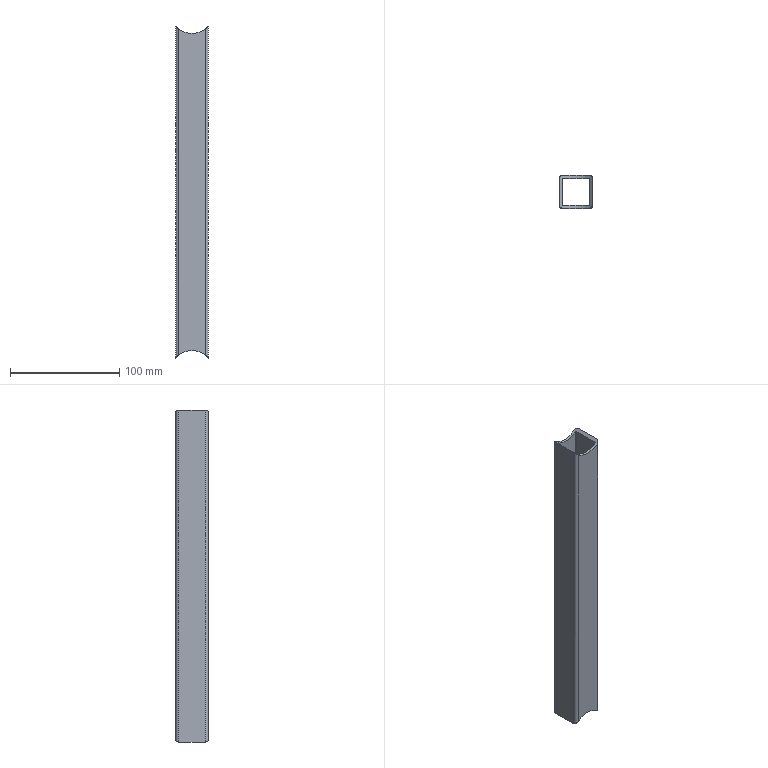Part | SolidWorks | features ExtruThin 1, ICE 1 | 1 solid | 19 faces | box 30 x 30 x 303.542 mm | volume 79870 mm3 | cylinder 11 | plane 8 | commonest cylinder face diameters 0.4 x4 5.4 x4 40 x3
STEP:
#1=CARTESIAN_POINT('',(0.,-15.,-145.));
#2=VERTEX_POINT('',#1);
#3=CARTESIAN_POINT('',(12.3,-15.,-149.229));
#4=VERTEX_POINT('',#3);
#5=CARTESIAN_POINT('',(0.,-15.,-165.));
#6=DIRECTION('',(0.,1.,0.));
#7=DIRECTION('',(0.,0.,1.));
#8=AXIS2_PLACEMENT_3D('',#5,#6,#7);
#9=CIRCLE('',#8,20.);
#10=EDGE_CURVE('',#2,#4,#9,.T.);
#11=ORIENTED_EDGE('',*,*,#10,.F.);
#12=CARTESIAN_POINT('',(0.,-12.5,-145.));
#13=VERTEX_POINT('',#12);
#14=CARTESIAN_POINT('',(0.,-25.,-145.));
#15=DIRECTION('',(0.,1.,0.));
#16=VECTOR('',#15,1000.);
#17=LINE('',#14,#16);
#18=EDGE_CURVE('',#2,#13,#17,.T.);
#19=ORIENTED_EDGE('',*,*,#18,.T.);
#20=CARTESIAN_POINT('',(12.3,-12.5,-149.229));
#21=VERTEX_POINT('',#20);
#22=CARTESIAN_POINT('',(0.,-12.5,-165.));
#23=DIRECTION('',(0.,1.,0.));
#24=DIRECTION('',(0.,0.,1.));
#25=AXIS2_PLACEMENT_3D('',#22,#23,#24);
#26=CIRCLE('',#25,20.);
#27=EDGE_CURVE('',#13,#21,#26,.T.);
#28=ORIENTED_EDGE('',*,*,#27,.T.);
#29=CARTESIAN_POINT('',(12.5,-12.3,-149.388));
#30=VERTEX_POINT('',#29);
#31=CARTESIAN_POINT('',(12.3,-12.5,-149.229));
#32=CARTESIAN_POINT('',(12.347,-12.5,-149.266));
#33=CARTESIAN_POINT('',(12.394,-12.484,-149.303));
#34=CARTESIAN_POINT('',(12.471,-12.416,-149.364));
#35=CARTESIAN_POINT('',(12.5,-12.36,-149.388));
#36=CARTESIAN_POINT('',(12.5,-12.3,-149.388));
#37=B_SPLINE_CURVE_WITH_KNOTS('',3,(#31,#32,#33,#34,#35,#36),.UNSPECIFIED.,.F.,.F.,(4,2,4),(0.0003546,0.0005332,0.0007119),.UNSPECIFIED.);
#38=EDGE_CURVE('',#21,#30,#37,.T.);
#39=ORIENTED_EDGE('',*,*,#38,.T.);
#40=CARTESIAN_POINT('',(12.5,12.3,-149.388));
#41=VERTEX_POINT('',#40);
#42=CARTESIAN_POINT('',(12.5,-25.,-149.388));
#43=DIRECTION('',(0.,1.,0.));
#44=VECTOR('',#43,1000.);
#45=LINE('',#42,#44);
#46=EDGE_CURVE('',#30,#41,#45,.T.);
#47=ORIENTED_EDGE('',*,*,#46,.T.);
#48=CARTESIAN_POINT('',(12.3,12.5,-149.229));
#49=VERTEX_POINT('',#48);
#50=CARTESIAN_POINT('',(12.5,12.3,-149.388));
#51=CARTESIAN_POINT('',(12.5,12.36,-149.388));
#52=CARTESIAN_POINT('',(12.471,12.416,-149.364));
#53=CARTESIAN_POINT('',(12.394,12.484,-149.303));
#54=CARTESIAN_POINT('',(12.347,12.5,-149.266));
#55=CARTESIAN_POINT('',(12.3,12.5,-149.229));
#56=B_SPLINE_CURVE_WITH_KNOTS('',3,(#50,#51,#52,#53,#54,#55),.UNSPECIFIED.,.F.,.F.,(4,2,4),(0.0007119,0.00089,0.001068),.UNSPECIFIED.);
#57=EDGE_CURVE('',#41,#49,#56,.T.);
#58=ORIENTED_EDGE('',*,*,#57,.T.);
#59=CARTESIAN_POINT('',(0.,12.5,-145.));
#60=VERTEX_POINT('',#59);
#61=CARTESIAN_POINT('',(0.,12.5,-165.));
#62=DIRECTION('',(0.,-1.,0.));
#63=DIRECTION('',(0.,0.,-1.));
#64=AXIS2_PLACEMENT_3D('',#61,#62,#63);
#65=CIRCLE('',#64,20.);
#66=EDGE_CURVE('',#49,#60,#65,.T.);
#67=ORIENTED_EDGE('',*,*,#66,.T.);
#68=CARTESIAN_POINT('',(0.,15.,-145.));
#69=VERTEX_POINT('',#68);
#70=CARTESIAN_POINT('',(0.,-25.,-145.));
#71=DIRECTION('',(0.,1.,0.));
#72=VECTOR('',#71,1000.);
#73=LINE('',#70,#72);
#74=EDGE_CURVE('',#60,#69,#73,.T.);
#75=ORIENTED_EDGE('',*,*,#74,.T.);
#76=CARTESIAN_POINT('',(12.3,15.,-149.229));
#77=VERTEX_POINT('',#76);
#78=CARTESIAN_POINT('',(0.,15.,-165.));
#79=DIRECTION('',(0.,-1.,0.));
#80=DIRECTION('',(0.,0.,-1.));
#81=AXIS2_PLACEMENT_3D('',#78,#79,#80);
#82=CIRCLE('',#81,20.);
#83=EDGE_CURVE('',#77,#69,#82,.T.);
#84=ORIENTED_EDGE('',*,*,#83,.F.);
#85=CARTESIAN_POINT('',(15.,12.3,-151.771));
#86=VERTEX_POINT('',#85);
#87=CARTESIAN_POINT('',(15.,12.3,-151.771));
#88=CARTESIAN_POINT('',(15.,12.512,-151.771));
#89=CARTESIAN_POINT('',(14.975,12.72,-151.743));
#90=CARTESIAN_POINT('',(14.881,13.119,-151.637));
#91=CARTESIAN_POINT('',(14.813,13.305,-151.562));
#92=CARTESIAN_POINT('',(14.647,13.649,-151.381));
#93=CARTESIAN_POINT('',(14.55,13.803,-151.277));
#94=CARTESIAN_POINT('',(14.335,14.084,-151.052));
#95=CARTESIAN_POINT('',(14.215,14.211,-150.93));
#96=CARTESIAN_POINT('',(13.964,14.433,-150.681));
#97=CARTESIAN_POINT('',(13.831,14.53,-150.552));
#98=CARTESIAN_POINT('',(13.552,14.698,-150.29));
#99=CARTESIAN_POINT('',(13.405,14.769,-150.156));
#100=CARTESIAN_POINT('',(13.102,14.883,-149.888));
#101=CARTESIAN_POINT('',(12.947,14.926,-149.755));
#102=CARTESIAN_POINT('',(12.63,14.985,-149.491));
#103=CARTESIAN_POINT('',(12.466,15.,-149.359));
#104=CARTESIAN_POINT('',(12.3,15.,-149.229));
#105=B_SPLINE_CURVE_WITH_KNOTS('',3,(#87,#88,#89,#90,#91,#92,#93,#94,#95,#96,#97,#98,#99,#100,#101,#102,#103,#104),.UNSPECIFIED.,.F.,.F.,(4,2,2,2,2,2,2,2,4),(0.00968,0.01031,0.01093,0.01156,0.01219,0.01281,0.01344,0.01407,0.01469),.UNSPECIFIED.);
#106=EDGE_CURVE('',#86,#77,#105,.T.);
#107=ORIENTED_EDGE('',*,*,#106,.F.);
#108=CARTESIAN_POINT('',(15.,-12.3,-151.771));
#109=VERTEX_POINT('',#108);
#110=CARTESIAN_POINT('',(15.,-25.,-151.771));
#111=DIRECTION('',(0.,1.,0.));
#112=VECTOR('',#111,1000.);
#113=LINE('',#110,#112);
#114=EDGE_CURVE('',#109,#86,#113,.T.);
#115=ORIENTED_EDGE('',*,*,#114,.F.);
#116=CARTESIAN_POINT('',(12.3,-15.,-149.229));
#117=CARTESIAN_POINT('',(12.466,-15.,-149.359));
#118=CARTESIAN_POINT('',(12.628,-14.985,-149.49));
#119=CARTESIAN_POINT('',(12.946,-14.926,-149.754));
#120=CARTESIAN_POINT('',(13.103,-14.883,-149.889));
#121=CARTESIAN_POINT('',(13.558,-14.711,-150.291));
#122=CARTESIAN_POINT('',(13.836,-14.546,-150.554));
#123=CARTESIAN_POINT('',(14.215,-14.21,-150.93));
#124=CARTESIAN_POINT('',(14.334,-14.084,-151.052));
#125=CARTESIAN_POINT('',(14.549,-13.804,-151.276));
#126=CARTESIAN_POINT('',(14.648,-13.647,-151.381));
#127=CARTESIAN_POINT('',(14.813,-13.305,-151.562));
#128=CARTESIAN_POINT('',(14.881,-13.12,-151.637));
#129=CARTESIAN_POINT('',(14.975,-12.72,-151.743));
#130=CARTESIAN_POINT('',(15.,-12.512,-151.771));
#131=CARTESIAN_POINT('',(15.,-12.3,-151.771));
#132=B_SPLINE_CURVE_WITH_KNOTS('',3,(#116,#117,#118,#119,#120,#121,#122,#123,#124,#125,#126,#127,#128,#129,#130,#131),.UNSPECIFIED.,.F.,.F.,(4,2,2,2,2,2,2,4),(0.004664,0.005291,0.005918,0.007172,0.007799,0.008426,0.009053,0.00968),.UNSPECIFIED.);
#133=EDGE_CURVE('',#4,#109,#132,.T.);
#134=ORIENTED_EDGE('',*,*,#133,.F.);
#135=EDGE_LOOP('',(#11,#19,#28,#39,#47,#58,#67,#75,#84,#107,#115,#134));
#136=FACE_OUTER_BOUND('',#135,.T.);
#137=CARTESIAN_POINT('',(0.,-25.,-165.));
#138=DIRECTION('',(0.,1.,0.));
#139=DIRECTION('',(0.,0.,1.));
#140=AXIS2_PLACEMENT_3D('',#137,#138,#139);
#141=CYLINDRICAL_SURFACE('',#140,20.);
#142=ADVANCED_FACE('',(#136),#141,.F.);
#143=CARTESIAN_POINT('',(-15.,-12.3,151.771));
#144=VERTEX_POINT('',#143);
#145=CARTESIAN_POINT('',(-15.,-12.3,-151.771));
#146=VERTEX_POINT('',#145);
#147=CARTESIAN_POINT('',(-15.,-12.3,165.));
#148=DIRECTION('',(0.,0.,-1.));
#149=VECTOR('',#148,1000.);
#150=LINE('',#147,#149);
#151=EDGE_CURVE('',#144,#146,#150,.T.);
#152=ORIENTED_EDGE('',*,*,#151,.T.);
#153=CARTESIAN_POINT('',(-12.3,-15.,-149.229));
#154=VERTEX_POINT('',#153);
#155=CARTESIAN_POINT('',(-15.,-12.3,-151.771));
#156=CARTESIAN_POINT('',(-15.,-12.513,-151.771));
#157=CARTESIAN_POINT('',(-14.975,-12.719,-151.743));
#158=CARTESIAN_POINT('',(-14.881,-13.117,-151.638));
#159=CARTESIAN_POINT('',(-14.814,-13.304,-151.562));
#160=CARTESIAN_POINT('',(-14.648,-13.647,-151.382));
#161=CARTESIAN_POINT('',(-14.549,-13.804,-151.276));
#162=CARTESIAN_POINT('',(-14.334,-14.084,-151.052));
#163=CARTESIAN_POINT('',(-14.216,-14.21,-150.931));
#164=CARTESIAN_POINT('',(-13.835,-14.547,-150.553));
#165=CARTESIAN_POINT('',(-13.557,-14.712,-150.29));
#166=CARTESIAN_POINT('',(-13.102,-14.883,-149.888));
#167=CARTESIAN_POINT('',(-12.945,-14.927,-149.753));
#168=CARTESIAN_POINT('',(-12.627,-14.985,-149.489));
#169=CARTESIAN_POINT('',(-12.465,-15.,-149.358));
#170=CARTESIAN_POINT('',(-12.3,-15.,-149.229));
#171=B_SPLINE_CURVE_WITH_KNOTS('',3,(#155,#156,#157,#158,#159,#160,#161,#162,#163,#164,#165,#166,#167,#168,#169,#170),.UNSPECIFIED.,.F.,.F.,(4,2,2,2,2,2,2,4),(0.,0.0006274,0.001255,0.001882,0.002509,0.003764,0.004391,0.005019),.UNSPECIFIED.);
#172=EDGE_CURVE('',#146,#154,#171,.T.);
#173=ORIENTED_EDGE('',*,*,#172,.T.);
#174=CARTESIAN_POINT('',(-12.3,-15.,149.229));
#175=VERTEX_POINT('',#174);
#176=CARTESIAN_POINT('',(-12.3,-15.,165.));
#177=DIRECTION('',(0.,0.,-1.));
#178=VECTOR('',#177,1000.);
#179=LINE('',#176,#178);
#180=EDGE_CURVE('',#175,#154,#179,.T.);
#181=ORIENTED_EDGE('',*,*,#180,.F.);
#182=CARTESIAN_POINT('',(-12.3,-15.,149.229));
#183=CARTESIAN_POINT('',(-12.633,-15.,149.489));
#184=CARTESIAN_POINT('',(-12.951,-14.94,149.754));
#185=CARTESIAN_POINT('',(-13.405,-14.769,150.156));
#186=CARTESIAN_POINT('',(-13.552,-14.698,150.29));
#187=CARTESIAN_POINT('',(-13.83,-14.53,150.551));
#188=CARTESIAN_POINT('',(-13.963,-14.434,150.679));
#189=CARTESIAN_POINT('',(-14.214,-14.212,150.929));
#190=CARTESIAN_POINT('',(-14.333,-14.085,151.051));
#191=CARTESIAN_POINT('',(-14.549,-13.804,151.276));
#192=CARTESIAN_POINT('',(-14.646,-13.65,151.38));
#193=CARTESIAN_POINT('',(-14.813,-13.305,151.562));
#194=CARTESIAN_POINT('',(-14.88,-13.121,151.637));
#195=CARTESIAN_POINT('',(-14.975,-12.723,151.742));
#196=CARTESIAN_POINT('',(-15.,-12.513,151.771));
#197=CARTESIAN_POINT('',(-15.,-12.3,151.771));
#198=B_SPLINE_CURVE_WITH_KNOTS('',3,(#182,#183,#184,#185,#186,#187,#188,#189,#190,#191,#192,#193,#194,#195,#196,#197),.UNSPECIFIED.,.F.,.F.,(4,2,2,2,2,2,2,4),(0.,0.001252,0.001878,0.002504,0.00313,0.003756,0.004382,0.005008),.UNSPECIFIED.);
#199=EDGE_CURVE('',#175,#144,#198,.T.);
#200=ORIENTED_EDGE('',*,*,#199,.T.);
#201=EDGE_LOOP('',(#152,#173,#181,#200));
#202=FACE_OUTER_BOUND('',#201,.T.);
#203=CARTESIAN_POINT('',(-12.3,-12.3,165.));
#204=DIRECTION('',(0.,0.,-1.));
#205=DIRECTION('',(-1.,0.,0.));
#206=AXIS2_PLACEMENT_3D('',#203,#204,#205);
#207=CYLINDRICAL_SURFACE('',#206,2.7);
#208=ADVANCED_FACE('',(#202),#207,.T.);
#209=ORIENTED_EDGE('',*,*,#180,.T.);
#210=CARTESIAN_POINT('',(0.,-15.,-165.));
#211=DIRECTION('',(0.,1.,0.));
#212=DIRECTION('',(0.,0.,1.));
#213=AXIS2_PLACEMENT_3D('',#210,#211,#212);
#214=CIRCLE('',#213,20.);
#215=EDGE_CURVE('',#154,#2,#214,.T.);
#216=ORIENTED_EDGE('',*,*,#215,.T.);
#217=ORIENTED_EDGE('',*,*,#10,.T.);
#218=CARTESIAN_POINT('',(12.3,-15.,149.229));
#219=VERTEX_POINT('',#218);
#220=CARTESIAN_POINT('',(12.3,-15.,165.));
#221=DIRECTION('',(0.,0.,-1.));
#222=VECTOR('',#221,1000.);
#223=LINE('',#220,#222);
#224=EDGE_CURVE('',#219,#4,#223,.T.);
#225=ORIENTED_EDGE('',*,*,#224,.F.);
#226=CARTESIAN_POINT('',(0.,-15.,165.));
#227=DIRECTION('',(0.,1.,0.));
#228=DIRECTION('',(0.,0.,1.));
#229=AXIS2_PLACEMENT_3D('',#226,#227,#228);
#230=CIRCLE('',#229,20.);
#231=EDGE_CURVE('',#219,#175,#230,.T.);
#232=ORIENTED_EDGE('',*,*,#231,.T.);
#233=EDGE_LOOP('',(#209,#216,#217,#225,#232));
#234=FACE_OUTER_BOUND('',#233,.T.);
#235=CARTESIAN_POINT('',(-12.3,-15.,165.));
#236=DIRECTION('',(0.,1.,0.));
#237=DIRECTION('',(0.,0.,1.));
#238=AXIS2_PLACEMENT_3D('',#235,#236,#237);
#239=PLANE('',#238);
#240=ADVANCED_FACE('',(#234),#239,.F.);
#241=ORIENTED_EDGE('',*,*,#224,.T.);
#242=ORIENTED_EDGE('',*,*,#133,.T.);
#243=CARTESIAN_POINT('',(15.,-12.3,151.771));
#244=VERTEX_POINT('',#243);
#245=CARTESIAN_POINT('',(15.,-12.3,165.));
#246=DIRECTION('',(0.,0.,-1.));
#247=VECTOR('',#246,1000.);
#248=LINE('',#245,#247);
#249=EDGE_CURVE('',#244,#109,#248,.T.);
#250=ORIENTED_EDGE('',*,*,#249,.F.);
#251=CARTESIAN_POINT('',(15.,-12.3,151.771));
#252=CARTESIAN_POINT('',(15.,-12.513,151.771));
#253=CARTESIAN_POINT('',(14.975,-12.718,151.743));
#254=CARTESIAN_POINT('',(14.882,-13.117,151.638));
#255=CARTESIAN_POINT('',(14.814,-13.303,151.563));
#256=CARTESIAN_POINT('',(14.648,-13.646,151.382));
#257=CARTESIAN_POINT('',(14.55,-13.803,151.277));
#258=CARTESIAN_POINT('',(14.336,-14.083,151.053));
#259=CARTESIAN_POINT('',(14.218,-14.208,150.933));
#260=CARTESIAN_POINT('',(13.837,-14.545,150.555));
#261=CARTESIAN_POINT('',(13.559,-14.71,150.293));
#262=CARTESIAN_POINT('',(13.105,-14.882,149.891));
#263=CARTESIAN_POINT('',(12.948,-14.926,149.756));
#264=CARTESIAN_POINT('',(12.629,-14.985,149.491));
#265=CARTESIAN_POINT('',(12.467,-15.,149.359));
#266=CARTESIAN_POINT('',(12.3,-15.,149.229));
#267=B_SPLINE_CURVE_WITH_KNOTS('',3,(#251,#252,#253,#254,#255,#256,#257,#258,#259,#260,#261,#262,#263,#264,#265,#266),.UNSPECIFIED.,.F.,.F.,(4,2,2,2,2,2,2,4),(0.,0.0006267,0.001253,0.00188,0.002507,0.00376,0.004387,0.005013),.UNSPECIFIED.);
#268=EDGE_CURVE('',#244,#219,#267,.T.);
#269=ORIENTED_EDGE('',*,*,#268,.T.);
#270=EDGE_LOOP('',(#241,#242,#250,#269));
#271=FACE_OUTER_BOUND('',#270,.T.);
#272=CARTESIAN_POINT('',(12.3,-12.3,165.));
#273=DIRECTION('',(0.,0.,-1.));
#274=DIRECTION('',(-1.,0.,0.));
#275=AXIS2_PLACEMENT_3D('',#272,#273,#274);
#276=CYLINDRICAL_SURFACE('',#275,2.7);
#277=ADVANCED_FACE('',(#271),#276,.T.);
#278=ORIENTED_EDGE('',*,*,#249,.T.);
#279=ORIENTED_EDGE('',*,*,#114,.T.);
#280=CARTESIAN_POINT('',(15.,12.3,151.771));
#281=VERTEX_POINT('',#280);
#282=CARTESIAN_POINT('',(15.,12.3,165.));
#283=DIRECTION('',(0.,0.,-1.));
#284=VECTOR('',#283,1000.);
#285=LINE('',#282,#284);
#286=EDGE_CURVE('',#281,#86,#285,.T.);
#287=ORIENTED_EDGE('',*,*,#286,.F.);
#288=CARTESIAN_POINT('',(15.,-25.,151.771));
#289=DIRECTION('',(0.,-1.,0.));
#290=VECTOR('',#289,1000.);
#291=LINE('',#288,#290);
#292=EDGE_CURVE('',#281,#244,#291,.T.);
#293=ORIENTED_EDGE('',*,*,#292,.T.);
#294=EDGE_LOOP('',(#278,#279,#287,#293));
#295=FACE_OUTER_BOUND('',#294,.T.);
#296=CARTESIAN_POINT('',(15.,12.3,165.));
#297=DIRECTION('',(-1.,0.,0.));
#298=DIRECTION('',(0.,0.,1.));
#299=AXIS2_PLACEMENT_3D('',#296,#297,#298);
#300=PLANE('',#299);
#301=ADVANCED_FACE('',(#295),#300,.F.);
#302=ORIENTED_EDGE('',*,*,#286,.T.);
#303=ORIENTED_EDGE('',*,*,#106,.T.);
#304=CARTESIAN_POINT('',(12.3,15.,149.229));
#305=VERTEX_POINT('',#304);
#306=CARTESIAN_POINT('',(12.3,15.,165.));
#307=DIRECTION('',(0.,0.,-1.));
#308=VECTOR('',#307,1000.);
#309=LINE('',#306,#308);
#310=EDGE_CURVE('',#305,#77,#309,.T.);
#311=ORIENTED_EDGE('',*,*,#310,.F.);
#312=CARTESIAN_POINT('',(12.3,15.,149.229));
#313=CARTESIAN_POINT('',(12.633,15.,149.489));
#314=CARTESIAN_POINT('',(12.951,14.94,149.754));
#315=CARTESIAN_POINT('',(13.405,14.769,150.156));
#316=CARTESIAN_POINT('',(13.552,14.698,150.29));
#317=CARTESIAN_POINT('',(13.83,14.53,150.551));
#318=CARTESIAN_POINT('',(13.963,14.434,150.679));
#319=CARTESIAN_POINT('',(14.214,14.212,150.929));
#320=CARTESIAN_POINT('',(14.333,14.085,151.051));
#321=CARTESIAN_POINT('',(14.549,13.804,151.276));
#322=CARTESIAN_POINT('',(14.646,13.65,151.38));
#323=CARTESIAN_POINT('',(14.813,13.305,151.562));
#324=CARTESIAN_POINT('',(14.88,13.121,151.637));
#325=CARTESIAN_POINT('',(14.975,12.723,151.742));
#326=CARTESIAN_POINT('',(15.,12.513,151.771));
#327=CARTESIAN_POINT('',(15.,12.3,151.771));
#328=B_SPLINE_CURVE_WITH_KNOTS('',3,(#312,#313,#314,#315,#316,#317,#318,#319,#320,#321,#322,#323,#324,#325,#326,#327),.UNSPECIFIED.,.F.,.F.,(4,2,2,2,2,2,2,4),(0.,0.001252,0.001878,0.002504,0.00313,0.003756,0.004382,0.005008),.UNSPECIFIED.);
#329=EDGE_CURVE('',#305,#281,#328,.T.);
#330=ORIENTED_EDGE('',*,*,#329,.T.);
#331=EDGE_LOOP('',(#302,#303,#311,#330));
#332=FACE_OUTER_BOUND('',#331,.T.);
#333=CARTESIAN_POINT('',(12.3,12.3,165.));
#334=DIRECTION('',(0.,0.,-1.));
#335=DIRECTION('',(-1.,0.,0.));
#336=AXIS2_PLACEMENT_3D('',#333,#334,#335);
#337=CYLINDRICAL_SURFACE('',#336,2.7);
#338=ADVANCED_FACE('',(#332),#337,.T.);
#339=ORIENTED_EDGE('',*,*,#310,.T.);
#340=ORIENTED_EDGE('',*,*,#83,.T.);
#341=CARTESIAN_POINT('',(-12.3,15.,-149.229));
#342=VERTEX_POINT('',#341);
#343=CARTESIAN_POINT('',(0.,15.,-165.));
#344=DIRECTION('',(0.,-1.,0.));
#345=DIRECTION('',(0.,0.,-1.));
#346=AXIS2_PLACEMENT_3D('',#343,#344,#345);
#347=CIRCLE('',#346,20.);
#348=EDGE_CURVE('',#69,#342,#347,.T.);
#349=ORIENTED_EDGE('',*,*,#348,.T.);
#350=CARTESIAN_POINT('',(-12.3,15.,149.229));
#351=VERTEX_POINT('',#350);
#352=CARTESIAN_POINT('',(-12.3,15.,165.));
#353=DIRECTION('',(0.,0.,-1.));
#354=VECTOR('',#353,1000.);
#355=LINE('',#352,#354);
#356=EDGE_CURVE('',#351,#342,#355,.T.);
#357=ORIENTED_EDGE('',*,*,#356,.F.);
#358=CARTESIAN_POINT('',(0.,15.,165.));
#359=DIRECTION('',(0.,-1.,0.));
#360=DIRECTION('',(0.,0.,-1.));
#361=AXIS2_PLACEMENT_3D('',#358,#359,#360);
#362=CIRCLE('',#361,20.);
#363=EDGE_CURVE('',#351,#305,#362,.T.);
#364=ORIENTED_EDGE('',*,*,#363,.T.);
#365=EDGE_LOOP('',(#339,#340,#349,#357,#364));
#366=FACE_OUTER_BOUND('',#365,.T.);
#367=CARTESIAN_POINT('',(-12.3,15.,165.));
#368=DIRECTION('',(0.,-1.,0.));
#369=DIRECTION('',(0.,0.,-1.));
#370=AXIS2_PLACEMENT_3D('',#367,#368,#369);
#371=PLANE('',#370);
#372=ADVANCED_FACE('',(#366),#371,.F.);
#373=ORIENTED_EDGE('',*,*,#356,.T.);
#374=CARTESIAN_POINT('',(-15.,12.3,-151.771));
#375=VERTEX_POINT('',#374);
#376=CARTESIAN_POINT('',(-12.3,15.,-149.229));
#377=CARTESIAN_POINT('',(-12.465,15.,-149.358));
#378=CARTESIAN_POINT('',(-12.627,14.985,-149.489));
#379=CARTESIAN_POINT('',(-12.947,14.926,-149.755));
#380=CARTESIAN_POINT('',(-13.104,14.882,-149.89));
#381=CARTESIAN_POINT('',(-13.405,14.769,-150.156));
#382=CARTESIAN_POINT('',(-13.55,14.699,-150.288));
#383=CARTESIAN_POINT('',(-13.829,14.531,-150.55));
#384=CARTESIAN_POINT('',(-13.964,14.433,-150.681));
#385=CARTESIAN_POINT('',(-14.216,14.21,-150.931));
#386=CARTESIAN_POINT('',(-14.333,14.085,-151.051));
#387=CARTESIAN_POINT('',(-14.549,13.804,-151.276));
#388=CARTESIAN_POINT('',(-14.647,13.647,-151.381));
#389=CARTESIAN_POINT('',(-14.812,13.307,-151.561));
#390=CARTESIAN_POINT('',(-14.881,13.119,-151.637));
#391=CARTESIAN_POINT('',(-14.974,12.723,-151.742));
#392=CARTESIAN_POINT('',(-15.,12.512,-151.771));
#393=CARTESIAN_POINT('',(-15.,12.3,-151.771));
#394=B_SPLINE_CURVE_WITH_KNOTS('',3,(#376,#377,#378,#379,#380,#381,#382,#383,#384,#385,#386,#387,#388,#389,#390,#391,#392,#393),.UNSPECIFIED.,.F.,.F.,(4,2,2,2,2,2,2,2,4),(0.01434,0.01497,0.01559,0.01622,0.01684,0.01747,0.01809,0.01872,0.01934),.UNSPECIFIED.);
#395=EDGE_CURVE('',#342,#375,#394,.T.);
#396=ORIENTED_EDGE('',*,*,#395,.T.);
#397=CARTESIAN_POINT('',(-15.,12.3,151.771));
#398=VERTEX_POINT('',#397);
#399=CARTESIAN_POINT('',(-15.,12.3,165.));
#400=DIRECTION('',(0.,0.,-1.));
#401=VECTOR('',#400,1000.);
#402=LINE('',#399,#401);
#403=EDGE_CURVE('',#398,#375,#402,.T.);
#404=ORIENTED_EDGE('',*,*,#403,.F.);
#405=CARTESIAN_POINT('',(-15.,12.3,151.771));
#406=CARTESIAN_POINT('',(-15.,12.513,151.771));
#407=CARTESIAN_POINT('',(-14.975,12.718,151.743));
#408=CARTESIAN_POINT('',(-14.882,13.117,151.638));
#409=CARTESIAN_POINT('',(-14.814,13.303,151.563));
#410=CARTESIAN_POINT('',(-14.648,13.646,151.382));
#411=CARTESIAN_POINT('',(-14.55,13.803,151.277));
#412=CARTESIAN_POINT('',(-14.336,14.083,151.053));
#413=CARTESIAN_POINT('',(-14.218,14.208,150.933));
#414=CARTESIAN_POINT('',(-13.837,14.545,150.555));
#415=CARTESIAN_POINT('',(-13.559,14.71,150.293));
#416=CARTESIAN_POINT('',(-13.105,14.882,149.891));
#417=CARTESIAN_POINT('',(-12.948,14.926,149.756));
#418=CARTESIAN_POINT('',(-12.629,14.985,149.491));
#419=CARTESIAN_POINT('',(-12.467,15.,149.359));
#420=CARTESIAN_POINT('',(-12.3,15.,149.229));
#421=B_SPLINE_CURVE_WITH_KNOTS('',3,(#405,#406,#407,#408,#409,#410,#411,#412,#413,#414,#415,#416,#417,#418,#419,#420),.UNSPECIFIED.,.F.,.F.,(4,2,2,2,2,2,2,4),(0.,0.0006267,0.001253,0.00188,0.002507,0.00376,0.004387,0.005013),.UNSPECIFIED.);
#422=EDGE_CURVE('',#398,#351,#421,.T.);
#423=ORIENTED_EDGE('',*,*,#422,.T.);
#424=EDGE_LOOP('',(#373,#396,#404,#423));
#425=FACE_OUTER_BOUND('',#424,.T.);
#426=CARTESIAN_POINT('',(-12.3,12.3,165.));
#427=DIRECTION('',(0.,0.,-1.));
#428=DIRECTION('',(-1.,0.,0.));
#429=AXIS2_PLACEMENT_3D('',#426,#427,#428);
#430=CYLINDRICAL_SURFACE('',#429,2.7);
#431=ADVANCED_FACE('',(#425),#430,.T.);
#432=ORIENTED_EDGE('',*,*,#403,.T.);
#433=CARTESIAN_POINT('',(-15.,-25.,-151.771));
#434=DIRECTION('',(0.,-1.,0.));
#435=VECTOR('',#434,1000.);
#436=LINE('',#433,#435);
#437=EDGE_CURVE('',#375,#146,#436,.T.);
#438=ORIENTED_EDGE('',*,*,#437,.T.);
#439=ORIENTED_EDGE('',*,*,#151,.F.);
#440=CARTESIAN_POINT('',(-15.,-25.,151.771));
#441=DIRECTION('',(0.,1.,0.));
#442=VECTOR('',#441,1000.);
#443=LINE('',#440,#442);
#444=EDGE_CURVE('',#144,#398,#443,.T.);
#445=ORIENTED_EDGE('',*,*,#444,.T.);
#446=EDGE_LOOP('',(#432,#438,#439,#445));
#447=FACE_OUTER_BOUND('',#446,.T.);
#448=CARTESIAN_POINT('',(-15.,12.3,165.));
#449=DIRECTION('',(1.,0.,0.));
#450=DIRECTION('',(0.,0.,-1.));
#451=AXIS2_PLACEMENT_3D('',#448,#449,#450);
#452=PLANE('',#451);
#453=ADVANCED_FACE('',(#447),#452,.F.);
#454=CARTESIAN_POINT('',(-12.5,-12.3,-149.388));
#455=VERTEX_POINT('',#454);
#456=CARTESIAN_POINT('',(-12.3,-12.5,-149.229));
#457=VERTEX_POINT('',#456);
#458=CARTESIAN_POINT('',(-12.5,-12.3,-149.388));
#459=CARTESIAN_POINT('',(-12.5,-12.36,-149.388));
#460=CARTESIAN_POINT('',(-12.471,-12.415,-149.365));
#461=CARTESIAN_POINT('',(-12.394,-12.484,-149.303));
#462=CARTESIAN_POINT('',(-12.347,-12.5,-149.266));
#463=CARTESIAN_POINT('',(-12.3,-12.5,-149.229));
#464=B_SPLINE_CURVE_WITH_KNOTS('',3,(#458,#459,#460,#461,#462,#463),.UNSPECIFIED.,.F.,.F.,(4,2,4),(0.,0.0001784,0.0003568),.UNSPECIFIED.);
#465=EDGE_CURVE('',#455,#457,#464,.T.);
#466=ORIENTED_EDGE('',*,*,#465,.F.);
#467=CARTESIAN_POINT('',(-12.5,-12.3,149.388));
#468=VERTEX_POINT('',#467);
#469=CARTESIAN_POINT('',(-12.5,-12.3,165.));
#470=DIRECTION('',(0.,0.,-1.));
#471=VECTOR('',#470,1000.);
#472=LINE('',#469,#471);
#473=EDGE_CURVE('',#468,#455,#472,.T.);
#474=ORIENTED_EDGE('',*,*,#473,.F.);
#475=CARTESIAN_POINT('',(-12.3,-12.5,149.229));
#476=VERTEX_POINT('',#475);
#477=CARTESIAN_POINT('',(-12.3,-12.5,149.229));
#478=CARTESIAN_POINT('',(-12.347,-12.5,149.266));
#479=CARTESIAN_POINT('',(-12.394,-12.484,149.303));
#480=CARTESIAN_POINT('',(-12.471,-12.416,149.364));
#481=CARTESIAN_POINT('',(-12.5,-12.36,149.388));
#482=CARTESIAN_POINT('',(-12.5,-12.3,149.388));
#483=B_SPLINE_CURVE_WITH_KNOTS('',3,(#477,#478,#479,#480,#481,#482),.UNSPECIFIED.,.F.,.F.,(4,2,4),(0.,0.000178,0.0003559),.UNSPECIFIED.);
#484=EDGE_CURVE('',#476,#468,#483,.T.);
#485=ORIENTED_EDGE('',*,*,#484,.F.);
#486=CARTESIAN_POINT('',(-12.3,-12.5,165.));
#487=DIRECTION('',(0.,0.,-1.));
#488=VECTOR('',#487,1000.);
#489=LINE('',#486,#488);
#490=EDGE_CURVE('',#476,#457,#489,.T.);
#491=ORIENTED_EDGE('',*,*,#490,.T.);
#492=EDGE_LOOP('',(#466,#474,#485,#491));
#493=FACE_OUTER_BOUND('',#492,.T.);
#494=CARTESIAN_POINT('',(-12.3,-12.3,165.));
#495=DIRECTION('',(0.,0.,-1.));
#496=DIRECTION('',(-1.,0.,0.));
#497=AXIS2_PLACEMENT_3D('',#494,#495,#496);
#498=CYLINDRICAL_SURFACE('',#497,0.2);
#499=ADVANCED_FACE('',(#493),#498,.F.);
#500=CARTESIAN_POINT('',(0.,-12.5,-165.));
#501=DIRECTION('',(0.,1.,0.));
#502=DIRECTION('',(0.,0.,1.));
#503=AXIS2_PLACEMENT_3D('',#500,#501,#502);
#504=CIRCLE('',#503,20.);
#505=EDGE_CURVE('',#457,#13,#504,.T.);
#506=ORIENTED_EDGE('',*,*,#505,.F.);
#507=ORIENTED_EDGE('',*,*,#490,.F.);
#508=CARTESIAN_POINT('',(12.3,-12.5,149.229));
#509=VERTEX_POINT('',#508);
#510=CARTESIAN_POINT('',(0.,-12.5,165.));
#511=DIRECTION('',(0.,1.,0.));
#512=DIRECTION('',(0.,0.,1.));
#513=AXIS2_PLACEMENT_3D('',#510,#511,#512);
#514=CIRCLE('',#513,20.);
#515=EDGE_CURVE('',#509,#476,#514,.T.);
#516=ORIENTED_EDGE('',*,*,#515,.F.);
#517=CARTESIAN_POINT('',(12.3,-12.5,165.));
#518=DIRECTION('',(0.,0.,-1.));
#519=VECTOR('',#518,1000.);
#520=LINE('',#517,#519);
#521=EDGE_CURVE('',#509,#21,#520,.T.);
#522=ORIENTED_EDGE('',*,*,#521,.T.);
#523=ORIENTED_EDGE('',*,*,#27,.F.);
#524=EDGE_LOOP('',(#506,#507,#516,#522,#523));
#525=FACE_OUTER_BOUND('',#524,.T.);
#526=CARTESIAN_POINT('',(-12.3,-12.5,165.));
#527=DIRECTION('',(0.,1.,0.));
#528=DIRECTION('',(0.,0.,1.));
#529=AXIS2_PLACEMENT_3D('',#526,#527,#528);
#530=PLANE('',#529);
#531=ADVANCED_FACE('',(#525),#530,.T.);
#532=ORIENTED_EDGE('',*,*,#38,.F.);
#533=ORIENTED_EDGE('',*,*,#521,.F.);
#534=CARTESIAN_POINT('',(12.5,-12.3,149.388));
#535=VERTEX_POINT('',#534);
#536=CARTESIAN_POINT('',(12.5,-12.3,149.388));
#537=CARTESIAN_POINT('',(12.5,-12.36,149.388));
#538=CARTESIAN_POINT('',(12.471,-12.415,149.365));
#539=CARTESIAN_POINT('',(12.394,-12.484,149.303));
#540=CARTESIAN_POINT('',(12.347,-12.5,149.266));
#541=CARTESIAN_POINT('',(12.3,-12.5,149.229));
#542=B_SPLINE_CURVE_WITH_KNOTS('',3,(#536,#537,#538,#539,#540,#541),.UNSPECIFIED.,.F.,.F.,(4,2,4),(0.,0.0001784,0.0003568),.UNSPECIFIED.);
#543=EDGE_CURVE('',#535,#509,#542,.T.);
#544=ORIENTED_EDGE('',*,*,#543,.F.);
#545=CARTESIAN_POINT('',(12.5,-12.3,165.));
#546=DIRECTION('',(0.,0.,-1.));
#547=VECTOR('',#546,1000.);
#548=LINE('',#545,#547);
#549=EDGE_CURVE('',#535,#30,#548,.T.);
#550=ORIENTED_EDGE('',*,*,#549,.T.);
#551=EDGE_LOOP('',(#532,#533,#544,#550));
#552=FACE_OUTER_BOUND('',#551,.T.);
#553=CARTESIAN_POINT('',(12.3,-12.3,165.));
#554=DIRECTION('',(0.,0.,-1.));
#555=DIRECTION('',(-1.,0.,0.));
#556=AXIS2_PLACEMENT_3D('',#553,#554,#555);
#557=CYLINDRICAL_SURFACE('',#556,0.2);
#558=ADVANCED_FACE('',(#552),#557,.F.);
#559=ORIENTED_EDGE('',*,*,#46,.F.);
#560=ORIENTED_EDGE('',*,*,#549,.F.);
#561=CARTESIAN_POINT('',(12.5,12.3,149.388));
#562=VERTEX_POINT('',#561);
#563=CARTESIAN_POINT('',(12.5,-25.,149.388));
#564=DIRECTION('',(0.,-1.,0.));
#565=VECTOR('',#564,1000.);
#566=LINE('',#563,#565);
#567=EDGE_CURVE('',#562,#535,#566,.T.);
#568=ORIENTED_EDGE('',*,*,#567,.F.);
#569=CARTESIAN_POINT('',(12.5,12.3,165.));
#570=DIRECTION('',(0.,0.,-1.));
#571=VECTOR('',#570,1000.);
#572=LINE('',#569,#571);
#573=EDGE_CURVE('',#562,#41,#572,.T.);
#574=ORIENTED_EDGE('',*,*,#573,.T.);
#575=EDGE_LOOP('',(#559,#560,#568,#574));
#576=FACE_OUTER_BOUND('',#575,.T.);
#577=CARTESIAN_POINT('',(12.5,12.3,165.));
#578=DIRECTION('',(-1.,0.,0.));
#579=DIRECTION('',(0.,0.,1.));
#580=AXIS2_PLACEMENT_3D('',#577,#578,#579);
#581=PLANE('',#580);
#582=ADVANCED_FACE('',(#576),#581,.T.);
#583=ORIENTED_EDGE('',*,*,#57,.F.);
#584=ORIENTED_EDGE('',*,*,#573,.F.);
#585=CARTESIAN_POINT('',(12.3,12.5,149.229));
#586=VERTEX_POINT('',#585);
#587=CARTESIAN_POINT('',(12.3,12.5,149.229));
#588=CARTESIAN_POINT('',(12.347,12.5,149.266));
#589=CARTESIAN_POINT('',(12.394,12.484,149.303));
#590=CARTESIAN_POINT('',(12.471,12.416,149.364));
#591=CARTESIAN_POINT('',(12.5,12.36,149.388));
#592=CARTESIAN_POINT('',(12.5,12.3,149.388));
#593=B_SPLINE_CURVE_WITH_KNOTS('',3,(#587,#588,#589,#590,#591,#592),.UNSPECIFIED.,.F.,.F.,(4,2,4),(0.,0.000178,0.0003559),.UNSPECIFIED.);
#594=EDGE_CURVE('',#586,#562,#593,.T.);
#595=ORIENTED_EDGE('',*,*,#594,.F.);
#596=CARTESIAN_POINT('',(12.3,12.5,165.));
#597=DIRECTION('',(0.,0.,-1.));
#598=VECTOR('',#597,1000.);
#599=LINE('',#596,#598);
#600=EDGE_CURVE('',#586,#49,#599,.T.);
#601=ORIENTED_EDGE('',*,*,#600,.T.);
#602=EDGE_LOOP('',(#583,#584,#595,#601));
#603=FACE_OUTER_BOUND('',#602,.T.);
#604=CARTESIAN_POINT('',(12.3,12.3,165.));
#605=DIRECTION('',(0.,0.,-1.));
#606=DIRECTION('',(-1.,0.,0.));
#607=AXIS2_PLACEMENT_3D('',#604,#605,#606);
#608=CYLINDRICAL_SURFACE('',#607,0.2);
#609=ADVANCED_FACE('',(#603),#608,.F.);
#610=ORIENTED_EDGE('',*,*,#66,.F.);
#611=ORIENTED_EDGE('',*,*,#600,.F.);
#612=CARTESIAN_POINT('',(-12.3,12.5,149.229));
#613=VERTEX_POINT('',#612);
#614=CARTESIAN_POINT('',(0.,12.5,165.));
#615=DIRECTION('',(0.,-1.,0.));
#616=DIRECTION('',(0.,0.,-1.));
#617=AXIS2_PLACEMENT_3D('',#614,#615,#616);
#618=CIRCLE('',#617,20.);
#619=EDGE_CURVE('',#613,#586,#618,.T.);
#620=ORIENTED_EDGE('',*,*,#619,.F.);
#621=CARTESIAN_POINT('',(-12.3,12.5,-149.229));
#622=VERTEX_POINT('',#621);
#623=CARTESIAN_POINT('',(-12.3,12.5,165.));
#624=DIRECTION('',(0.,0.,-1.));
#625=VECTOR('',#624,1000.);
#626=LINE('',#623,#625);
#627=EDGE_CURVE('',#613,#622,#626,.T.);
#628=ORIENTED_EDGE('',*,*,#627,.T.);
#629=CARTESIAN_POINT('',(0.,12.5,-165.));
#630=DIRECTION('',(0.,-1.,0.));
#631=DIRECTION('',(0.,0.,-1.));
#632=AXIS2_PLACEMENT_3D('',#629,#630,#631);
#633=CIRCLE('',#632,20.);
#634=EDGE_CURVE('',#60,#622,#633,.T.);
#635=ORIENTED_EDGE('',*,*,#634,.F.);
#636=EDGE_LOOP('',(#610,#611,#620,#628,#635));
#637=FACE_OUTER_BOUND('',#636,.T.);
#638=CARTESIAN_POINT('',(-12.3,12.5,165.));
#639=DIRECTION('',(0.,-1.,0.));
#640=DIRECTION('',(0.,0.,-1.));
#641=AXIS2_PLACEMENT_3D('',#638,#639,#640);
#642=PLANE('',#641);
#643=ADVANCED_FACE('',(#637),#642,.T.);
#644=CARTESIAN_POINT('',(-12.5,12.3,-149.388));
#645=VERTEX_POINT('',#644);
#646=CARTESIAN_POINT('',(-12.3,12.5,-149.229));
#647=CARTESIAN_POINT('',(-12.347,12.5,-149.266));
#648=CARTESIAN_POINT('',(-12.394,12.484,-149.303));
#649=CARTESIAN_POINT('',(-12.471,12.416,-149.364));
#650=CARTESIAN_POINT('',(-12.5,12.36,-149.388));
#651=CARTESIAN_POINT('',(-12.5,12.3,-149.388));
#652=B_SPLINE_CURVE_WITH_KNOTS('',3,(#646,#647,#648,#649,#650,#651),.UNSPECIFIED.,.F.,.F.,(4,2,4),(0.001066,0.001244,0.001423),.UNSPECIFIED.);
#653=EDGE_CURVE('',#622,#645,#652,.T.);
#654=ORIENTED_EDGE('',*,*,#653,.F.);
#655=ORIENTED_EDGE('',*,*,#627,.F.);
#656=CARTESIAN_POINT('',(-12.5,12.3,149.388));
#657=VERTEX_POINT('',#656);
#658=CARTESIAN_POINT('',(-12.5,12.3,149.388));
#659=CARTESIAN_POINT('',(-12.5,12.36,149.388));
#660=CARTESIAN_POINT('',(-12.471,12.415,149.365));
#661=CARTESIAN_POINT('',(-12.394,12.484,149.303));
#662=CARTESIAN_POINT('',(-12.347,12.5,149.266));
#663=CARTESIAN_POINT('',(-12.3,12.5,149.229));
#664=B_SPLINE_CURVE_WITH_KNOTS('',3,(#658,#659,#660,#661,#662,#663),.UNSPECIFIED.,.F.,.F.,(4,2,4),(0.,0.0001784,0.0003568),.UNSPECIFIED.);
#665=EDGE_CURVE('',#657,#613,#664,.T.);
#666=ORIENTED_EDGE('',*,*,#665,.F.);
#667=CARTESIAN_POINT('',(-12.5,12.3,165.));
#668=DIRECTION('',(0.,0.,-1.));
#669=VECTOR('',#668,1000.);
#670=LINE('',#667,#669);
#671=EDGE_CURVE('',#657,#645,#670,.T.);
#672=ORIENTED_EDGE('',*,*,#671,.T.);
#673=EDGE_LOOP('',(#654,#655,#666,#672));
#674=FACE_OUTER_BOUND('',#673,.T.);
#675=CARTESIAN_POINT('',(-12.3,12.3,165.));
#676=DIRECTION('',(0.,0.,-1.));
#677=DIRECTION('',(-1.,0.,0.));
#678=AXIS2_PLACEMENT_3D('',#675,#676,#677);
#679=CYLINDRICAL_SURFACE('',#678,0.2);
#680=ADVANCED_FACE('',(#674),#679,.F.);
#681=CARTESIAN_POINT('',(-12.5,-25.,-149.388));
#682=DIRECTION('',(0.,-1.,0.));
#683=VECTOR('',#682,1000.);
#684=LINE('',#681,#683);
#685=EDGE_CURVE('',#645,#455,#684,.T.);
#686=ORIENTED_EDGE('',*,*,#685,.F.);
#687=ORIENTED_EDGE('',*,*,#671,.F.);
#688=CARTESIAN_POINT('',(-12.5,-25.,149.388));
#689=DIRECTION('',(0.,1.,0.));
#690=VECTOR('',#689,1000.);
#691=LINE('',#688,#690);
#692=EDGE_CURVE('',#468,#657,#691,.T.);
#693=ORIENTED_EDGE('',*,*,#692,.F.);
#694=ORIENTED_EDGE('',*,*,#473,.T.);
#695=EDGE_LOOP('',(#686,#687,#693,#694));
#696=FACE_OUTER_BOUND('',#695,.T.);
#697=CARTESIAN_POINT('',(-12.5,12.3,165.));
#698=DIRECTION('',(1.,0.,0.));
#699=DIRECTION('',(0.,0.,-1.));
#700=AXIS2_PLACEMENT_3D('',#697,#698,#699);
#701=PLANE('',#700);
#702=ADVANCED_FACE('',(#696),#701,.T.);
#703=ORIENTED_EDGE('',*,*,#484,.T.);
#704=ORIENTED_EDGE('',*,*,#692,.T.);
#705=ORIENTED_EDGE('',*,*,#665,.T.);
#706=ORIENTED_EDGE('',*,*,#619,.T.);
#707=ORIENTED_EDGE('',*,*,#594,.T.);
#708=ORIENTED_EDGE('',*,*,#567,.T.);
#709=ORIENTED_EDGE('',*,*,#543,.T.);
#710=ORIENTED_EDGE('',*,*,#515,.T.);
#711=EDGE_LOOP('',(#703,#704,#705,#706,#707,#708,#709,#710));
#712=FACE_BOUND('',#711,.T.);
#713=ORIENTED_EDGE('',*,*,#231,.F.);
#714=ORIENTED_EDGE('',*,*,#268,.F.);
#715=ORIENTED_EDGE('',*,*,#292,.F.);
#716=ORIENTED_EDGE('',*,*,#329,.F.);
#717=ORIENTED_EDGE('',*,*,#363,.F.);
#718=ORIENTED_EDGE('',*,*,#422,.F.);
#719=ORIENTED_EDGE('',*,*,#444,.F.);
#720=ORIENTED_EDGE('',*,*,#199,.F.);
#721=EDGE_LOOP('',(#713,#714,#715,#716,#717,#718,#719,#720));
#722=FACE_OUTER_BOUND('',#721,.T.);
#723=CARTESIAN_POINT('',(0.,-25.,165.));
#724=DIRECTION('',(0.,1.,0.));
#725=DIRECTION('',(0.,0.,1.));
#726=AXIS2_PLACEMENT_3D('',#723,#724,#725);
#727=CYLINDRICAL_SURFACE('',#726,20.);
#728=ADVANCED_FACE('',(#712,#722),#727,.F.);
#729=ORIENTED_EDGE('',*,*,#18,.F.);
#730=ORIENTED_EDGE('',*,*,#215,.F.);
#731=ORIENTED_EDGE('',*,*,#172,.F.);
#732=ORIENTED_EDGE('',*,*,#437,.F.);
#733=ORIENTED_EDGE('',*,*,#395,.F.);
#734=ORIENTED_EDGE('',*,*,#348,.F.);
#735=ORIENTED_EDGE('',*,*,#74,.F.);
#736=ORIENTED_EDGE('',*,*,#634,.T.);
#737=ORIENTED_EDGE('',*,*,#653,.T.);
#738=ORIENTED_EDGE('',*,*,#685,.T.);
#739=ORIENTED_EDGE('',*,*,#465,.T.);
#740=ORIENTED_EDGE('',*,*,#505,.T.);
#741=EDGE_LOOP('',(#729,#730,#731,#732,#733,#734,#735,#736,#737,#738,#739,#740));
#742=FACE_OUTER_BOUND('',#741,.T.);
#743=CARTESIAN_POINT('',(0.,-25.,-165.));
#744=DIRECTION('',(0.,1.,0.));
#745=DIRECTION('',(0.,0.,1.));
#746=AXIS2_PLACEMENT_3D('',#743,#744,#745);
#747=CYLINDRICAL_SURFACE('',#746,20.);
#748=ADVANCED_FACE('',(#742),#747,.F.);
#749=CLOSED_SHELL('',(#142,#208,#240,#277,#301,#338,#372,#431,#453,#499,#531,#558,#582,#609,#643,#680,#702,#728,#748));
#750=MANIFOLD_SOLID_BREP('',#749);
#751=CARTESIAN_POINT('',(0.,0.,0.));
#752=DIRECTION('',(0.,0.,1.));
#753=DIRECTION('',(1.,0.,0.));
#754=AXIS2_PLACEMENT_3D('',#751,#752,#753);
#755=(LENGTH_UNIT()NAMED_UNIT(*)SI_UNIT(.MILLI.,.METRE.));
#756=UNCERTAINTY_MEASURE_WITH_UNIT(LENGTH_MEASURE(0.00001),#755,'','');
#757=(NAMED_UNIT(*)PLANE_ANGLE_UNIT()SI_UNIT($,.RADIAN.));
#758=(NAMED_UNIT(*)SI_UNIT($,.STERADIAN.)SOLID_ANGLE_UNIT());
#759=(GEOMETRIC_REPRESENTATION_CONTEXT(3)GLOBAL_UNCERTAINTY_ASSIGNED_CONTEXT((#756))GLOBAL_UNIT_ASSIGNED_CONTEXT((#755,#757,#758))REPRESENTATION_CONTEXT('',''));
#760=ADVANCED_BREP_SHAPE_REPRESENTATION('',(#750,#754),#759);